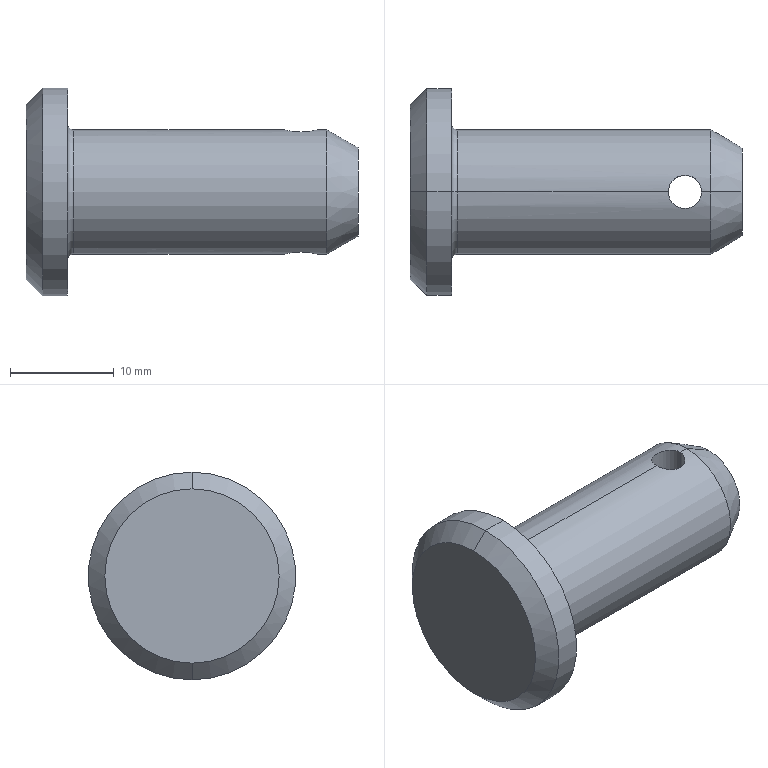Part | SolidWorks | features MBimport 1 | 1 solid | 15 faces | box 32 x 20 x 20 mm | volume 4166 mm3 | cylinder 6 | cone 4 | plane 3 | torus 2 | commonest cylinder face diameters 3.2 x2 12 x2 20 x2
STEP:
#1=CARTESIAN_POINT('',(32.,0.,-4.268));
#2=VERTEX_POINT('',#1);
#3=CARTESIAN_POINT('',(29.,0.,-6.));
#4=VERTEX_POINT('',#3);
#5=CARTESIAN_POINT('',(32.,0.,-4.268));
#6=DIRECTION('',(-0.866,0.,-0.5));
#7=VECTOR('',#6,1000.);
#8=LINE('',#5,#7);
#9=EDGE_CURVE('',#2,#4,#8,.T.);
#10=ORIENTED_EDGE('',*,*,#9,.F.);
#11=CARTESIAN_POINT('',(32.,0.,4.268));
#12=VERTEX_POINT('',#11);
#13=CARTESIAN_POINT('',(32.,0.,0.));
#14=DIRECTION('',(1.,0.,0.));
#15=DIRECTION('',(0.,0.,-1.));
#16=AXIS2_PLACEMENT_3D('',#13,#14,#15);
#17=CIRCLE('',#16,4.268);
#18=EDGE_CURVE('',#12,#2,#17,.T.);
#19=ORIENTED_EDGE('',*,*,#18,.F.);
#20=CARTESIAN_POINT('',(29.,0.,6.));
#21=VERTEX_POINT('',#20);
#22=CARTESIAN_POINT('',(32.,0.,4.268));
#23=DIRECTION('',(-0.866,0.,0.5));
#24=VECTOR('',#23,1000.);
#25=LINE('',#22,#24);
#26=EDGE_CURVE('',#12,#21,#25,.T.);
#27=ORIENTED_EDGE('',*,*,#26,.T.);
#28=CARTESIAN_POINT('',(29.,0.,0.));
#29=DIRECTION('',(-1.,0.,0.));
#30=DIRECTION('',(0.,0.,-1.));
#31=AXIS2_PLACEMENT_3D('',#28,#29,#30);
#32=CIRCLE('',#31,6.);
#33=EDGE_CURVE('',#4,#21,#32,.T.);
#34=ORIENTED_EDGE('',*,*,#33,.F.);
#35=EDGE_LOOP('',(#10,#19,#27,#34));
#36=FACE_OUTER_BOUND('',#35,.T.);
#37=CARTESIAN_POINT('',(32.,0.,0.));
#38=DIRECTION('',(-1.,0.,0.));
#39=DIRECTION('',(0.,0.,1.));
#40=AXIS2_PLACEMENT_3D('',#37,#38,#39);
#41=CONICAL_SURFACE('',#40,4.268,0.5236);
#42=ADVANCED_FACE('',(#36),#41,.T.);
#43=CARTESIAN_POINT('',(4.6,0.,6.));
#44=VERTEX_POINT('',#43);
#45=CARTESIAN_POINT('',(4.,0.,6.6));
#46=VERTEX_POINT('',#45);
#47=CARTESIAN_POINT('',(4.6,0.,6.6));
#48=DIRECTION('',(0.,1.,0.));
#49=DIRECTION('',(0.,0.,1.));
#50=AXIS2_PLACEMENT_3D('',#47,#48,#49);
#51=CIRCLE('',#50,0.6);
#52=EDGE_CURVE('',#44,#46,#51,.T.);
#53=ORIENTED_EDGE('',*,*,#52,.F.);
#54=CARTESIAN_POINT('',(4.6,0.,-6.));
#55=VERTEX_POINT('',#54);
#56=CARTESIAN_POINT('',(4.6,0.,0.));
#57=DIRECTION('',(1.,0.,0.));
#58=DIRECTION('',(0.,0.,-1.));
#59=AXIS2_PLACEMENT_3D('',#56,#57,#58);
#60=CIRCLE('',#59,6.);
#61=EDGE_CURVE('',#55,#44,#60,.T.);
#62=ORIENTED_EDGE('',*,*,#61,.F.);
#63=CARTESIAN_POINT('',(4.,0.,-6.6));
#64=VERTEX_POINT('',#63);
#65=CARTESIAN_POINT('',(4.6,0.,-6.6));
#66=DIRECTION('',(0.,-1.,0.));
#67=DIRECTION('',(0.,0.,-1.));
#68=AXIS2_PLACEMENT_3D('',#65,#66,#67);
#69=CIRCLE('',#68,0.6);
#70=EDGE_CURVE('',#55,#64,#69,.T.);
#71=ORIENTED_EDGE('',*,*,#70,.T.);
#72=CARTESIAN_POINT('',(4.,0.,0.));
#73=DIRECTION('',(-1.,0.,0.));
#74=DIRECTION('',(0.,0.,-1.));
#75=AXIS2_PLACEMENT_3D('',#72,#73,#74);
#76=CIRCLE('',#75,6.6);
#77=EDGE_CURVE('',#46,#64,#76,.T.);
#78=ORIENTED_EDGE('',*,*,#77,.F.);
#79=EDGE_LOOP('',(#53,#62,#71,#78));
#80=FACE_OUTER_BOUND('',#79,.T.);
#81=CARTESIAN_POINT('',(4.6,0.,0.));
#82=DIRECTION('',(1.,0.,0.));
#83=DIRECTION('',(0.,0.,-1.));
#84=AXIS2_PLACEMENT_3D('',#81,#82,#83);
#85=TOROIDAL_SURFACE('',#84,6.6,0.6);
#86=ADVANCED_FACE('',(#80),#85,.F.);
#87=CARTESIAN_POINT('',(24.9,0.,-6.));
#88=VERTEX_POINT('',#87);
#89=CARTESIAN_POINT('',(24.9,0.,6.));
#90=VERTEX_POINT('',#89);
#91=CARTESIAN_POINT('',(24.9,0.,-10.));
#92=DIRECTION('',(0.,0.,1.));
#93=VECTOR('',#92,1000.);
#94=LINE('',#91,#93);
#95=EDGE_CURVE('',#88,#90,#94,.T.);
#96=ORIENTED_EDGE('',*,*,#95,.F.);
#97=CARTESIAN_POINT('',(28.1,0.,-6.));
#98=VERTEX_POINT('',#97);
#99=CARTESIAN_POINT('',(24.9,0.,-6.));
#100=CARTESIAN_POINT('',(24.9,0.1062,-6.));
#101=CARTESIAN_POINT('',(24.91,0.2105,-5.997));
#102=CARTESIAN_POINT('',(24.951,0.4156,-5.986));
#103=CARTESIAN_POINT('',(24.982,0.5175,-5.978));
#104=CARTESIAN_POINT('',(25.063,0.711,-5.959));
#105=CARTESIAN_POINT('',(25.112,0.8027,-5.947));
#106=CARTESIAN_POINT('',(25.228,0.9763,-5.921));
#107=CARTESIAN_POINT('',(25.295,1.058,-5.906));
#108=CARTESIAN_POINT('',(25.516,1.278,-5.864));
#109=CARTESIAN_POINT('',(25.693,1.397,-5.836));
#110=CARTESIAN_POINT('',(26.078,1.557,-5.795));
#111=CARTESIAN_POINT('',(26.289,1.6,-5.783));
#112=CARTESIAN_POINT('',(26.603,1.6,-5.783));
#113=CARTESIAN_POINT('',(26.71,1.59,-5.786));
#114=CARTESIAN_POINT('',(26.915,1.549,-5.797));
#115=CARTESIAN_POINT('',(27.015,1.518,-5.805));
#116=CARTESIAN_POINT('',(27.307,1.398,-5.836));
#117=CARTESIAN_POINT('',(27.483,1.28,-5.864));
#118=CARTESIAN_POINT('',(27.705,1.058,-5.906));
#119=CARTESIAN_POINT('',(27.771,0.9778,-5.92));
#120=CARTESIAN_POINT('',(27.887,0.805,-5.946));
#121=CARTESIAN_POINT('',(27.937,0.7113,-5.958));
#122=CARTESIAN_POINT('',(28.057,0.4219,-5.988));
#123=CARTESIAN_POINT('',(28.1,0.2124,-6.));
#124=CARTESIAN_POINT('',(28.1,0.,-6.));
#125=B_SPLINE_CURVE_WITH_KNOTS('',3,(#99,#100,#101,#102,#103,#104,#105,#106,#107,#108,#109,#110,#111,#112,#113,#114,#115,#116,#117,#118,#119,#120,#121,#122,#123,#124),.UNSPECIFIED.,.F.,.F.,(4,2,2,2,2,2,2,2,2,2,2,2,4),(0.,0.000314,0.0006279,0.0009419,0.001256,0.001884,0.002512,0.002826,0.00314,0.003768,0.004082,0.004396,0.005024),.UNSPECIFIED.);
#126=EDGE_CURVE('',#88,#98,#125,.T.);
#127=ORIENTED_EDGE('',*,*,#126,.T.);
#128=CARTESIAN_POINT('',(28.1,0.,6.));
#129=VERTEX_POINT('',#128);
#130=CARTESIAN_POINT('',(28.1,0.,-10.));
#131=DIRECTION('',(0.,0.,1.));
#132=VECTOR('',#131,1000.);
#133=LINE('',#130,#132);
#134=EDGE_CURVE('',#98,#129,#133,.T.);
#135=ORIENTED_EDGE('',*,*,#134,.T.);
#136=CARTESIAN_POINT('',(28.1,0.,6.));
#137=CARTESIAN_POINT('',(28.1,0.1062,6.));
#138=CARTESIAN_POINT('',(28.09,0.2105,5.997));
#139=CARTESIAN_POINT('',(28.049,0.4156,5.986));
#140=CARTESIAN_POINT('',(28.018,0.5175,5.978));
#141=CARTESIAN_POINT('',(27.937,0.711,5.959));
#142=CARTESIAN_POINT('',(27.888,0.8027,5.947));
#143=CARTESIAN_POINT('',(27.772,0.9763,5.921));
#144=CARTESIAN_POINT('',(27.705,1.058,5.906));
#145=CARTESIAN_POINT('',(27.484,1.278,5.864));
#146=CARTESIAN_POINT('',(27.307,1.397,5.836));
#147=CARTESIAN_POINT('',(26.922,1.557,5.795));
#148=CARTESIAN_POINT('',(26.711,1.6,5.783));
#149=CARTESIAN_POINT('',(26.397,1.6,5.783));
#150=CARTESIAN_POINT('',(26.29,1.59,5.786));
#151=CARTESIAN_POINT('',(26.085,1.549,5.797));
#152=CARTESIAN_POINT('',(25.985,1.518,5.805));
#153=CARTESIAN_POINT('',(25.693,1.398,5.836));
#154=CARTESIAN_POINT('',(25.517,1.28,5.864));
#155=CARTESIAN_POINT('',(25.295,1.058,5.906));
#156=CARTESIAN_POINT('',(25.229,0.9778,5.92));
#157=CARTESIAN_POINT('',(25.113,0.805,5.946));
#158=CARTESIAN_POINT('',(25.063,0.7113,5.958));
#159=CARTESIAN_POINT('',(24.943,0.4219,5.988));
#160=CARTESIAN_POINT('',(24.9,0.2124,6.));
#161=CARTESIAN_POINT('',(24.9,0.,6.));
#162=B_SPLINE_CURVE_WITH_KNOTS('',3,(#136,#137,#138,#139,#140,#141,#142,#143,#144,#145,#146,#147,#148,#149,#150,#151,#152,#153,#154,#155,#156,#157,#158,#159,#160,#161),.UNSPECIFIED.,.F.,.F.,(4,2,2,2,2,2,2,2,2,2,2,2,4),(0.,0.000314,0.0006279,0.0009419,0.001256,0.001884,0.002512,0.002826,0.00314,0.003768,0.004082,0.004396,0.005024),.UNSPECIFIED.);
#163=EDGE_CURVE('',#129,#90,#162,.T.);
#164=ORIENTED_EDGE('',*,*,#163,.T.);
#165=EDGE_LOOP('',(#96,#127,#135,#164));
#166=FACE_OUTER_BOUND('',#165,.T.);
#167=CARTESIAN_POINT('',(26.5,0.,-10.));
#168=DIRECTION('',(0.,0.,1.));
#169=DIRECTION('',(1.,0.,0.));
#170=AXIS2_PLACEMENT_3D('',#167,#168,#169);
#171=CYLINDRICAL_SURFACE('',#170,1.6);
#172=ADVANCED_FACE('',(#166),#171,.F.);
#173=ORIENTED_EDGE('',*,*,#18,.T.);
#174=CARTESIAN_POINT('',(32.,0.,0.));
#175=DIRECTION('',(1.,0.,0.));
#176=DIRECTION('',(0.,0.,-1.));
#177=AXIS2_PLACEMENT_3D('',#174,#175,#176);
#178=CIRCLE('',#177,4.268);
#179=EDGE_CURVE('',#2,#12,#178,.T.);
#180=ORIENTED_EDGE('',*,*,#179,.T.);
#181=EDGE_LOOP('',(#173,#180));
#182=FACE_OUTER_BOUND('',#181,.T.);
#183=CARTESIAN_POINT('',(32.,6.,0.));
#184=DIRECTION('',(1.,0.,0.));
#185=DIRECTION('',(0.,1.,0.));
#186=AXIS2_PLACEMENT_3D('',#183,#184,#185);
#187=PLANE('',#186);
#188=ADVANCED_FACE('',(#182),#187,.T.);
#189=CARTESIAN_POINT('',(0.,0.,6.));
#190=DIRECTION('',(1.,0.,0.));
#191=VECTOR('',#190,1000.);
#192=LINE('',#189,#191);
#193=EDGE_CURVE('',#44,#90,#192,.T.);
#194=ORIENTED_EDGE('',*,*,#193,.F.);
#195=CARTESIAN_POINT('',(4.6,0.,0.));
#196=DIRECTION('',(1.,0.,0.));
#197=DIRECTION('',(0.,0.,-1.));
#198=AXIS2_PLACEMENT_3D('',#195,#196,#197);
#199=CIRCLE('',#198,6.);
#200=EDGE_CURVE('',#44,#55,#199,.T.);
#201=ORIENTED_EDGE('',*,*,#200,.T.);
#202=CARTESIAN_POINT('',(0.,0.,-6.));
#203=DIRECTION('',(1.,0.,0.));
#204=VECTOR('',#203,1000.);
#205=LINE('',#202,#204);
#206=EDGE_CURVE('',#55,#88,#205,.T.);
#207=ORIENTED_EDGE('',*,*,#206,.T.);
#208=CARTESIAN_POINT('',(28.1,0.,-6.));
#209=CARTESIAN_POINT('',(28.1,-0.1062,-6.));
#210=CARTESIAN_POINT('',(28.09,-0.2105,-5.997));
#211=CARTESIAN_POINT('',(28.049,-0.4156,-5.986));
#212=CARTESIAN_POINT('',(28.018,-0.5175,-5.978));
#213=CARTESIAN_POINT('',(27.937,-0.711,-5.959));
#214=CARTESIAN_POINT('',(27.888,-0.8027,-5.947));
#215=CARTESIAN_POINT('',(27.772,-0.9763,-5.921));
#216=CARTESIAN_POINT('',(27.705,-1.058,-5.906));
#217=CARTESIAN_POINT('',(27.484,-1.278,-5.864));
#218=CARTESIAN_POINT('',(27.307,-1.397,-5.836));
#219=CARTESIAN_POINT('',(26.922,-1.557,-5.795));
#220=CARTESIAN_POINT('',(26.711,-1.6,-5.783));
#221=CARTESIAN_POINT('',(26.397,-1.6,-5.783));
#222=CARTESIAN_POINT('',(26.29,-1.59,-5.786));
#223=CARTESIAN_POINT('',(26.085,-1.549,-5.797));
#224=CARTESIAN_POINT('',(25.985,-1.518,-5.805));
#225=CARTESIAN_POINT('',(25.693,-1.398,-5.836));
#226=CARTESIAN_POINT('',(25.517,-1.28,-5.864));
#227=CARTESIAN_POINT('',(25.295,-1.058,-5.906));
#228=CARTESIAN_POINT('',(25.229,-0.9778,-5.92));
#229=CARTESIAN_POINT('',(25.113,-0.805,-5.946));
#230=CARTESIAN_POINT('',(25.063,-0.7113,-5.958));
#231=CARTESIAN_POINT('',(24.943,-0.4219,-5.988));
#232=CARTESIAN_POINT('',(24.9,-0.2124,-6.));
#233=CARTESIAN_POINT('',(24.9,0.,-6.));
#234=B_SPLINE_CURVE_WITH_KNOTS('',3,(#208,#209,#210,#211,#212,#213,#214,#215,#216,#217,#218,#219,#220,#221,#222,#223,#224,#225,#226,#227,#228,#229,#230,#231,#232,#233),.UNSPECIFIED.,.F.,.F.,(4,2,2,2,2,2,2,2,2,2,2,2,4),(0.,0.000314,0.0006279,0.0009419,0.001256,0.001884,0.002512,0.002826,0.00314,0.003768,0.004082,0.004396,0.005024),.UNSPECIFIED.);
#235=EDGE_CURVE('',#98,#88,#234,.T.);
#236=ORIENTED_EDGE('',*,*,#235,.F.);
#237=CARTESIAN_POINT('',(0.,0.,-6.));
#238=DIRECTION('',(1.,0.,0.));
#239=VECTOR('',#238,1000.);
#240=LINE('',#237,#239);
#241=EDGE_CURVE('',#98,#4,#240,.T.);
#242=ORIENTED_EDGE('',*,*,#241,.T.);
#243=ORIENTED_EDGE('',*,*,#33,.T.);
#244=CARTESIAN_POINT('',(0.,0.,6.));
#245=DIRECTION('',(1.,0.,0.));
#246=VECTOR('',#245,1000.);
#247=LINE('',#244,#246);
#248=EDGE_CURVE('',#129,#21,#247,.T.);
#249=ORIENTED_EDGE('',*,*,#248,.F.);
#250=CARTESIAN_POINT('',(24.9,0.,6.));
#251=CARTESIAN_POINT('',(24.9,-0.1062,6.));
#252=CARTESIAN_POINT('',(24.91,-0.2105,5.997));
#253=CARTESIAN_POINT('',(24.951,-0.4156,5.986));
#254=CARTESIAN_POINT('',(24.982,-0.5175,5.978));
#255=CARTESIAN_POINT('',(25.063,-0.711,5.959));
#256=CARTESIAN_POINT('',(25.112,-0.8027,5.947));
#257=CARTESIAN_POINT('',(25.228,-0.9763,5.921));
#258=CARTESIAN_POINT('',(25.295,-1.058,5.906));
#259=CARTESIAN_POINT('',(25.516,-1.278,5.864));
#260=CARTESIAN_POINT('',(25.693,-1.397,5.836));
#261=CARTESIAN_POINT('',(26.078,-1.557,5.795));
#262=CARTESIAN_POINT('',(26.289,-1.6,5.783));
#263=CARTESIAN_POINT('',(26.603,-1.6,5.783));
#264=CARTESIAN_POINT('',(26.71,-1.59,5.786));
#265=CARTESIAN_POINT('',(26.915,-1.549,5.797));
#266=CARTESIAN_POINT('',(27.015,-1.518,5.805));
#267=CARTESIAN_POINT('',(27.307,-1.398,5.836));
#268=CARTESIAN_POINT('',(27.483,-1.28,5.864));
#269=CARTESIAN_POINT('',(27.705,-1.058,5.906));
#270=CARTESIAN_POINT('',(27.771,-0.9778,5.92));
#271=CARTESIAN_POINT('',(27.887,-0.805,5.946));
#272=CARTESIAN_POINT('',(27.937,-0.7113,5.958));
#273=CARTESIAN_POINT('',(28.057,-0.4219,5.988));
#274=CARTESIAN_POINT('',(28.1,-0.2124,6.));
#275=CARTESIAN_POINT('',(28.1,0.,6.));
#276=B_SPLINE_CURVE_WITH_KNOTS('',3,(#250,#251,#252,#253,#254,#255,#256,#257,#258,#259,#260,#261,#262,#263,#264,#265,#266,#267,#268,#269,#270,#271,#272,#273,#274,#275),.UNSPECIFIED.,.F.,.F.,(4,2,2,2,2,2,2,2,2,2,2,2,4),(0.,0.000314,0.0006279,0.0009419,0.001256,0.001884,0.002512,0.002826,0.00314,0.003768,0.004082,0.004396,0.005024),.UNSPECIFIED.);
#277=EDGE_CURVE('',#90,#129,#276,.T.);
#278=ORIENTED_EDGE('',*,*,#277,.F.);
#279=EDGE_LOOP('',(#194,#201,#207,#236,#242,#243,#249,#278));
#280=FACE_OUTER_BOUND('',#279,.T.);
#281=CARTESIAN_POINT('',(0.,0.,0.));
#282=DIRECTION('',(1.,0.,0.));
#283=DIRECTION('',(0.,0.,-1.));
#284=AXIS2_PLACEMENT_3D('',#281,#282,#283);
#285=CYLINDRICAL_SURFACE('',#284,6.);
#286=ADVANCED_FACE('',(#280),#285,.T.);
#287=CARTESIAN_POINT('',(4.,0.,0.));
#288=DIRECTION('',(-1.,0.,0.));
#289=DIRECTION('',(0.,0.,-1.));
#290=AXIS2_PLACEMENT_3D('',#287,#288,#289);
#291=CIRCLE('',#290,6.6);
#292=EDGE_CURVE('',#64,#46,#291,.T.);
#293=ORIENTED_EDGE('',*,*,#292,.T.);
#294=ORIENTED_EDGE('',*,*,#77,.T.);
#295=EDGE_LOOP('',(#293,#294));
#296=FACE_BOUND('',#295,.T.);
#297=CARTESIAN_POINT('',(4.,0.,-10.));
#298=VERTEX_POINT('',#297);
#299=CARTESIAN_POINT('',(4.,0.,10.));
#300=VERTEX_POINT('',#299);
#301=CARTESIAN_POINT('',(4.,0.,0.));
#302=DIRECTION('',(1.,0.,0.));
#303=DIRECTION('',(0.,0.,-1.));
#304=AXIS2_PLACEMENT_3D('',#301,#302,#303);
#305=CIRCLE('',#304,10.);
#306=EDGE_CURVE('',#298,#300,#305,.T.);
#307=ORIENTED_EDGE('',*,*,#306,.T.);
#308=CARTESIAN_POINT('',(4.,0.,0.));
#309=DIRECTION('',(1.,0.,0.));
#310=DIRECTION('',(0.,0.,-1.));
#311=AXIS2_PLACEMENT_3D('',#308,#309,#310);
#312=CIRCLE('',#311,10.);
#313=EDGE_CURVE('',#300,#298,#312,.T.);
#314=ORIENTED_EDGE('',*,*,#313,.T.);
#315=EDGE_LOOP('',(#307,#314));
#316=FACE_OUTER_BOUND('',#315,.T.);
#317=CARTESIAN_POINT('',(4.,10.,0.));
#318=DIRECTION('',(1.,0.,0.));
#319=DIRECTION('',(0.,1.,0.));
#320=AXIS2_PLACEMENT_3D('',#317,#318,#319);
#321=PLANE('',#320);
#322=ADVANCED_FACE('',(#296,#316),#321,.T.);
#323=CARTESIAN_POINT('',(1.6,0.,10.));
#324=VERTEX_POINT('',#323);
#325=CARTESIAN_POINT('',(0.,0.,10.));
#326=DIRECTION('',(1.,0.,0.));
#327=VECTOR('',#326,1000.);
#328=LINE('',#325,#327);
#329=EDGE_CURVE('',#324,#300,#328,.T.);
#330=ORIENTED_EDGE('',*,*,#329,.F.);
#331=CARTESIAN_POINT('',(1.6,0.,-10.));
#332=VERTEX_POINT('',#331);
#333=CARTESIAN_POINT('',(1.6,0.,0.));
#334=DIRECTION('',(1.,0.,0.));
#335=DIRECTION('',(0.,0.,-1.));
#336=AXIS2_PLACEMENT_3D('',#333,#334,#335);
#337=CIRCLE('',#336,10.);
#338=EDGE_CURVE('',#324,#332,#337,.T.);
#339=ORIENTED_EDGE('',*,*,#338,.T.);
#340=CARTESIAN_POINT('',(0.,0.,-10.));
#341=DIRECTION('',(1.,0.,0.));
#342=VECTOR('',#341,1000.);
#343=LINE('',#340,#342);
#344=EDGE_CURVE('',#332,#298,#343,.T.);
#345=ORIENTED_EDGE('',*,*,#344,.T.);
#346=ORIENTED_EDGE('',*,*,#313,.F.);
#347=EDGE_LOOP('',(#330,#339,#345,#346));
#348=FACE_OUTER_BOUND('',#347,.T.);
#349=CARTESIAN_POINT('',(0.,0.,0.));
#350=DIRECTION('',(1.,0.,0.));
#351=DIRECTION('',(0.,0.,-1.));
#352=AXIS2_PLACEMENT_3D('',#349,#350,#351);
#353=CYLINDRICAL_SURFACE('',#352,10.);
#354=ADVANCED_FACE('',(#348),#353,.T.);
#355=CARTESIAN_POINT('',(0.,0.,8.4));
#356=VERTEX_POINT('',#355);
#357=CARTESIAN_POINT('',(1.6,0.,10.));
#358=DIRECTION('',(0.7071,0.,0.7071));
#359=VECTOR('',#358,1000.);
#360=LINE('',#357,#359);
#361=EDGE_CURVE('',#356,#324,#360,.T.);
#362=ORIENTED_EDGE('',*,*,#361,.F.);
#363=CARTESIAN_POINT('',(0.,0.,-8.4));
#364=VERTEX_POINT('',#363);
#365=CARTESIAN_POINT('',(0.,0.,0.));
#366=DIRECTION('',(1.,0.,0.));
#367=DIRECTION('',(0.,0.,-1.));
#368=AXIS2_PLACEMENT_3D('',#365,#366,#367);
#369=CIRCLE('',#368,8.4);
#370=EDGE_CURVE('',#356,#364,#369,.T.);
#371=ORIENTED_EDGE('',*,*,#370,.T.);
#372=CARTESIAN_POINT('',(1.6,0.,-10.));
#373=DIRECTION('',(0.7071,0.,-0.7071));
#374=VECTOR('',#373,1000.);
#375=LINE('',#372,#374);
#376=EDGE_CURVE('',#364,#332,#375,.T.);
#377=ORIENTED_EDGE('',*,*,#376,.T.);
#378=ORIENTED_EDGE('',*,*,#338,.F.);
#379=EDGE_LOOP('',(#362,#371,#377,#378));
#380=FACE_OUTER_BOUND('',#379,.T.);
#381=CARTESIAN_POINT('',(1.6,0.,0.));
#382=DIRECTION('',(1.,0.,0.));
#383=DIRECTION('',(0.,0.,-1.));
#384=AXIS2_PLACEMENT_3D('',#381,#382,#383);
#385=CONICAL_SURFACE('',#384,10.,0.7854);
#386=ADVANCED_FACE('',(#380),#385,.T.);
#387=CARTESIAN_POINT('',(0.,0.,0.));
#388=DIRECTION('',(1.,0.,0.));
#389=DIRECTION('',(0.,0.,-1.));
#390=AXIS2_PLACEMENT_3D('',#387,#388,#389);
#391=CIRCLE('',#390,8.4);
#392=EDGE_CURVE('',#364,#356,#391,.T.);
#393=ORIENTED_EDGE('',*,*,#392,.F.);
#394=ORIENTED_EDGE('',*,*,#370,.F.);
#395=EDGE_LOOP('',(#393,#394));
#396=FACE_OUTER_BOUND('',#395,.T.);
#397=CARTESIAN_POINT('',(0.,0.,0.));
#398=DIRECTION('',(-1.,0.,0.));
#399=DIRECTION('',(0.,0.,1.));
#400=AXIS2_PLACEMENT_3D('',#397,#398,#399);
#401=PLANE('',#400);
#402=ADVANCED_FACE('',(#396),#401,.T.);
#403=ORIENTED_EDGE('',*,*,#392,.T.);
#404=ORIENTED_EDGE('',*,*,#361,.T.);
#405=CARTESIAN_POINT('',(1.6,0.,0.));
#406=DIRECTION('',(1.,0.,0.));
#407=DIRECTION('',(0.,0.,-1.));
#408=AXIS2_PLACEMENT_3D('',#405,#406,#407);
#409=CIRCLE('',#408,10.);
#410=EDGE_CURVE('',#332,#324,#409,.T.);
#411=ORIENTED_EDGE('',*,*,#410,.F.);
#412=ORIENTED_EDGE('',*,*,#376,.F.);
#413=EDGE_LOOP('',(#403,#404,#411,#412));
#414=FACE_OUTER_BOUND('',#413,.T.);
#415=CARTESIAN_POINT('',(1.6,0.,0.));
#416=DIRECTION('',(1.,0.,0.));
#417=DIRECTION('',(0.,0.,-1.));
#418=AXIS2_PLACEMENT_3D('',#415,#416,#417);
#419=CONICAL_SURFACE('',#418,10.,0.7854);
#420=ADVANCED_FACE('',(#414),#419,.T.);
#421=ORIENTED_EDGE('',*,*,#410,.T.);
#422=ORIENTED_EDGE('',*,*,#329,.T.);
#423=ORIENTED_EDGE('',*,*,#306,.F.);
#424=ORIENTED_EDGE('',*,*,#344,.F.);
#425=EDGE_LOOP('',(#421,#422,#423,#424));
#426=FACE_OUTER_BOUND('',#425,.T.);
#427=CARTESIAN_POINT('',(0.,0.,0.));
#428=DIRECTION('',(1.,0.,0.));
#429=DIRECTION('',(0.,0.,-1.));
#430=AXIS2_PLACEMENT_3D('',#427,#428,#429);
#431=CYLINDRICAL_SURFACE('',#430,10.);
#432=ADVANCED_FACE('',(#426),#431,.T.);
#433=ORIENTED_EDGE('',*,*,#61,.T.);
#434=ORIENTED_EDGE('',*,*,#193,.T.);
#435=ORIENTED_EDGE('',*,*,#163,.F.);
#436=ORIENTED_EDGE('',*,*,#248,.T.);
#437=CARTESIAN_POINT('',(29.,0.,0.));
#438=DIRECTION('',(-1.,0.,0.));
#439=DIRECTION('',(0.,0.,-1.));
#440=AXIS2_PLACEMENT_3D('',#437,#438,#439);
#441=CIRCLE('',#440,6.);
#442=EDGE_CURVE('',#21,#4,#441,.T.);
#443=ORIENTED_EDGE('',*,*,#442,.T.);
#444=ORIENTED_EDGE('',*,*,#241,.F.);
#445=ORIENTED_EDGE('',*,*,#126,.F.);
#446=ORIENTED_EDGE('',*,*,#206,.F.);
#447=EDGE_LOOP('',(#433,#434,#435,#436,#443,#444,#445,#446));
#448=FACE_OUTER_BOUND('',#447,.T.);
#449=CARTESIAN_POINT('',(0.,0.,0.));
#450=DIRECTION('',(1.,0.,0.));
#451=DIRECTION('',(0.,0.,-1.));
#452=AXIS2_PLACEMENT_3D('',#449,#450,#451);
#453=CYLINDRICAL_SURFACE('',#452,6.);
#454=ADVANCED_FACE('',(#448),#453,.T.);
#455=ORIENTED_EDGE('',*,*,#235,.T.);
#456=ORIENTED_EDGE('',*,*,#95,.T.);
#457=ORIENTED_EDGE('',*,*,#277,.T.);
#458=ORIENTED_EDGE('',*,*,#134,.F.);
#459=EDGE_LOOP('',(#455,#456,#457,#458));
#460=FACE_OUTER_BOUND('',#459,.T.);
#461=CARTESIAN_POINT('',(26.5,0.,-10.));
#462=DIRECTION('',(0.,0.,1.));
#463=DIRECTION('',(1.,0.,0.));
#464=AXIS2_PLACEMENT_3D('',#461,#462,#463);
#465=CYLINDRICAL_SURFACE('',#464,1.6);
#466=ADVANCED_FACE('',(#460),#465,.F.);
#467=ORIENTED_EDGE('',*,*,#200,.F.);
#468=ORIENTED_EDGE('',*,*,#52,.T.);
#469=ORIENTED_EDGE('',*,*,#292,.F.);
#470=ORIENTED_EDGE('',*,*,#70,.F.);
#471=EDGE_LOOP('',(#467,#468,#469,#470));
#472=FACE_OUTER_BOUND('',#471,.T.);
#473=CARTESIAN_POINT('',(4.6,0.,0.));
#474=DIRECTION('',(1.,0.,0.));
#475=DIRECTION('',(0.,0.,-1.));
#476=AXIS2_PLACEMENT_3D('',#473,#474,#475);
#477=TOROIDAL_SURFACE('',#476,6.6,0.6);
#478=ADVANCED_FACE('',(#472),#477,.F.);
#479=ORIENTED_EDGE('',*,*,#179,.F.);
#480=ORIENTED_EDGE('',*,*,#9,.T.);
#481=ORIENTED_EDGE('',*,*,#442,.F.);
#482=ORIENTED_EDGE('',*,*,#26,.F.);
#483=EDGE_LOOP('',(#479,#480,#481,#482));
#484=FACE_OUTER_BOUND('',#483,.T.);
#485=CARTESIAN_POINT('',(32.,0.,0.));
#486=DIRECTION('',(-1.,0.,0.));
#487=DIRECTION('',(0.,0.,1.));
#488=AXIS2_PLACEMENT_3D('',#485,#486,#487);
#489=CONICAL_SURFACE('',#488,4.268,0.5236);
#490=ADVANCED_FACE('',(#484),#489,.T.);
#491=CLOSED_SHELL('',(#42,#86,#172,#188,#286,#322,#354,#386,#402,#420,#432,#454,#466,#478,#490));
#492=MANIFOLD_SOLID_BREP('',#491);
#493=CARTESIAN_POINT('',(0.,0.,0.));
#494=DIRECTION('',(0.,0.,1.));
#495=DIRECTION('',(1.,0.,0.));
#496=AXIS2_PLACEMENT_3D('',#493,#494,#495);
#497=(LENGTH_UNIT()NAMED_UNIT(*)SI_UNIT(.MILLI.,.METRE.));
#498=UNCERTAINTY_MEASURE_WITH_UNIT(LENGTH_MEASURE(0.00001),#497,'','');
#499=(NAMED_UNIT(*)PLANE_ANGLE_UNIT()SI_UNIT($,.RADIAN.));
#500=(NAMED_UNIT(*)SI_UNIT($,.STERADIAN.)SOLID_ANGLE_UNIT());
#501=(GEOMETRIC_REPRESENTATION_CONTEXT(3)GLOBAL_UNCERTAINTY_ASSIGNED_CONTEXT((#498))GLOBAL_UNIT_ASSIGNED_CONTEXT((#497,#499,#500))REPRESENTATION_CONTEXT('',''));
#502=ADVANCED_BREP_SHAPE_REPRESENTATION('',(#492,#496),#501);